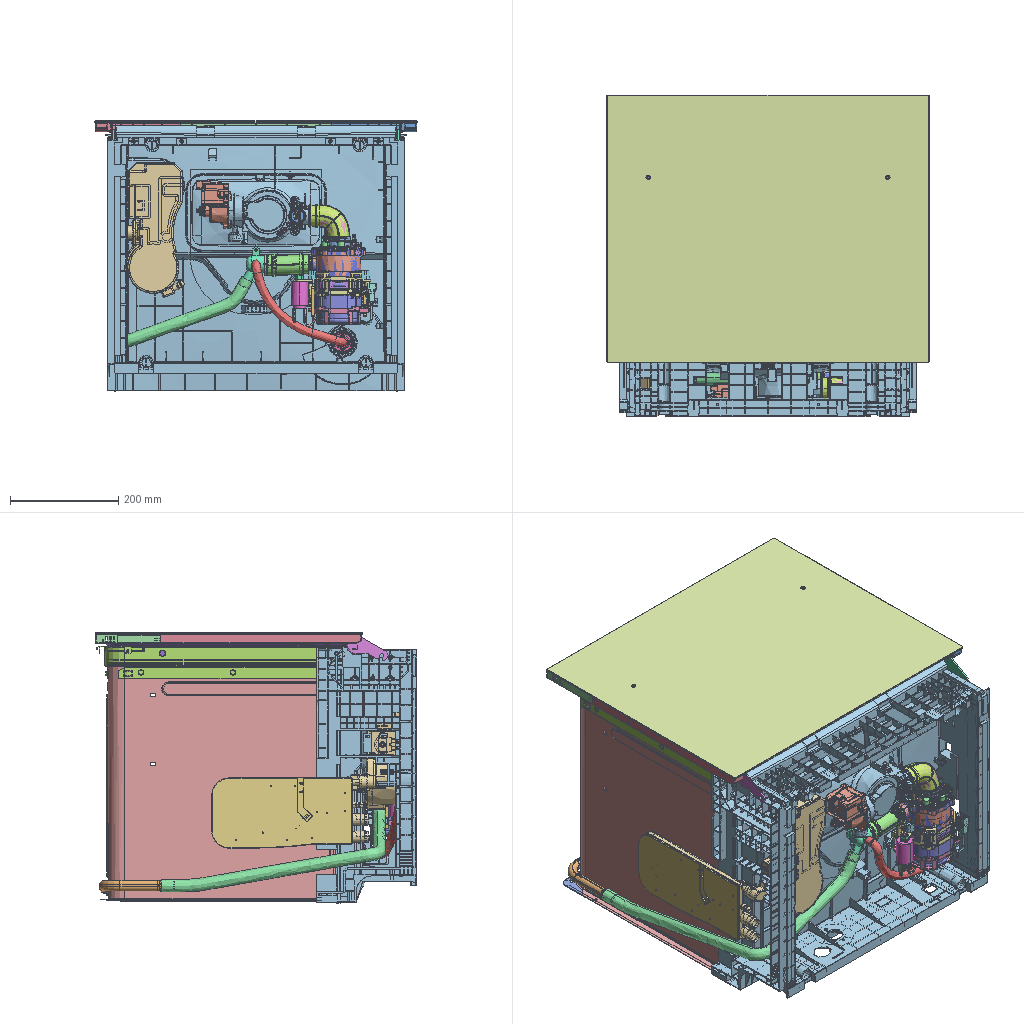Assembly | STEP file | 191 different items | 356 placed | box 596 x 594 x 500 mm
Parts list (item | name | quantity | parent item | size | volume):
1 | - | x1 | - | 3.8 x 3 x 1.2 mm | 13.052 mm3
2 | 12M0-U000-0002_A2512WRO-4P_1 | x1 | - | 12.48 x 9.8 x 8.57 mm | 221.308 mm3
3 | 12_12-3_5 | x1 | in BENGKEZUJIAN_ASM_29_ASM_1_ASM_1_ASM | 51.9 x 85 x 119.75 mm | 69599 mm3
4 | 19-HG_7_1 | x1 | in AC0410-190121_ASM_8_ASM_1_ASM | 112.641 x 83.966 x 33.2 mm | 28942 mm3
5 | 1903-QG_1 | x1 | in AC190301_ASM_2_ASM | 140.055 x 83.966 x 33 mm | 30398 mm3
6 | 8_20_3_1_1_14 | x1 | in BENGKEZUJIAN_ASM_29_ASM_1_ASM_1_ASM | 50.6 x 85 x 119.75 mm | 65552 mm3
7 | BENG1118_AF0_35_2_1_1 | x1 | in AC0410_ASM_9_ASM_6_ASM_3_ASM_1_ASM | 81.69 x 126.25 x 55 mm | 61777 mm3
8 | CHIWA_5_1_2_1_1 | x6 | in ZHUANZIZHUJIAN_ASM_9_1_ASM_1_AS_ASM | 18 x 11.5 x 2.4 mm | 490.68 mm3
9 | CIHUAN_7_1 | x1 | - | 34.75 x 20 x 34.75 mm | 14830 mm3
10 | DINGZITIEXING_8_1 | x1 | in ZHONGZHUANG_ASM_92_ASM_1_ASM | 73 x 15 x 73 mm | 38126 mm3
11 | DIZUO-XIN | x1 | in W721-DIZUO_ASM | - | 2428763 mm3
12 | DW-T1-02-0032_2_1_1 | x1 | in DW-T1-02-A004_ASM_1_ASM_2_ASM_1_ASM | 56 x 5.906 x 56 mm | 3121 mm3
13 | DW-T1-02-0033_2_6_1 | x1 | in DW-T1-02-A004_ASM_1_ASM_2_ASM_1_ASM | 56 x 19.052 x 56 mm | 7855 mm3
14 | DXDZ_1_1_1_1 | x1 | in AC0410_ASM_9_ASM_6_ASM_3_ASM_1_ASM | 8 x 16.965 x 7.531 mm | 100.473 mm3
15 | DZ250_3_1_1_1 | x2 | in AC0410_ASM_9_ASM_6_ASM_3_ASM_1_ASM | 8 x 13.602 x 13.602 mm | 104.298 mm3
16 | DZH_7_1 | x1 | - | 18.5 x 23 x 16 mm | 1219 mm3
17 | FANGHUALUOMAO_3_1 | x4 | in JIAREPANZUJIAN_ASM_76_ASM_2_ASM | 8 x 3.5 x 8 mm | 99.012 mm3
18 | GUANLU-XIAOPENBI | x1 | in 00-ZXW721_ASM_ASM | 176 x 160.5 x 71.93 mm | 30798 mm3
19 | HOUGAI_15_4 | x1 | in ZHONGZHUANG_ASM_92_ASM_1_ASM | 115 x 30 x 75 mm | 16947 mm3
20 | JAIREIPAN_146_1_1 | x1 | in JAIREIPAN_146_ASM_1_ASM | 99.5 x 85 x 6.5 mm | 5367 mm3
21 | JAIREIPAN_146_2_1 | x1 | in JAIREIPAN_146_ASM_1_ASM | 4.269 x 5.62 x 10.8 mm | 52.218 mm3
22 | JAIREIPAN_146_3_1 | x1 | in JAIREIPAN_146_ASM_1_ASM | 2.708 x 6.239 x 10.8 mm | 52.218 mm3
23 | JD20180502_ASM_1_ASM_2_1_1 | x1 | in DJ1118_ASM_5_ASM_4_ASM_7_ASM_1_ASM | - | -
24 | JD_1_1_1_1 | x2 | in DJ1118_ASM_5_ASM_4_ASM_7_ASM_1_ASM | 56 x 40 x 6 mm | 7974 mm3
25 | JIAREIGUAN_56_1 | x1 | in JIAREPANZUJIAN_ASM_76_ASM_2_ASM | 65 x 41.193 x 66.044 mm | 10951 mm3
26 | JIAREQI_2_1_1_1 | x1 | in AC0410_ASM_9_ASM_6_ASM_3_ASM_1_ASM | 62.5 x 63.088 x 35 mm | 12336 mm3
27 | LIANJIEQI1_17_1 | x1 | in ZHONGZHUANG_ASM_92_ASM_1_ASM | 19.4 x 30.7 x 11 mm | 1115 mm3
28 | LIANJIEQI2_14_1 | x1 | in ZHONGZHUANG_ASM_92_ASM_1_ASM | 20 x 23.5 x 10.5 mm | 729.279 mm3
29 | LUODING_1_1 | x6 | in JIAREPANZUJIAN_ASM_76_ASM_2_ASM | 6.44 x 6.44 x 10.399 mm | 92.165 mm3
30 | LUODING_1_1_1_1 | x4 | in DJ1118_ASM_5_ASM_4_ASM_7_ASM_1_ASM | - | -
31 | LUODING_5_1 | x3 | in ZHONGZHUANG_ASM_92_ASM_1_ASM | 5 x 14 x 5 mm | 98.522 mm3
32 | MIFENGQUAN1 | x1 | in 00-ZXW721_ASM_ASM | 19 x 19 x 3 mm | 355.306 mm3
33 | MIFENGQUAN2 | x1 | in 00-ZXW721_ASM_ASM | 28.5 x 28.5 x 2.6 mm | 525.838 mm3
34 | MIFENGQUAN_14_1_1_1 | x1 | in BENGKEZUJIAN_ASM_29_ASM_1_ASM_1_ASM | 81.15 x 81.15 x 2.65 mm | 1360 mm3
35 | MSBR-1 | x1 | in SHANGGEJIABAIFANG_ASM_ASM | 12.49 x 29.5 x 29.5 mm | 3348 mm3
36 | MSBR-10 | x1 | in SHANGGEJIABAIFANG_ASM_ASM | 12.49 x 29.5 x 29.5 mm | 3348 mm3
37 | MSBR-10_1_1_1_1 | x1 | in DJ1118_ASM_5_ASM_4_ASM_7_ASM_1_ASM | 7.904 x 7.691 x 3.2 mm | 92.564 mm3
38 | MSBR-11 | x1 | in SHANGGEJIABAIFANG_ASM_ASM | 26 x 13.7 x 15.65 mm | 1729 mm3
39 | MSBR-11_1_1_1_1 | x1 | in DJ1118_ASM_5_ASM_4_ASM_7_ASM_1_ASM | 7.691 x 7.904 x 3.2 mm | 92.564 mm3
40 | MSBR-12 | x1 | in SHANGGEJIABAIFANG_ASM_ASM | 12.744 x 31.5 x 31.5 mm | 3459 mm3
41 | MSBR-12_1_1_1_1 | x1 | in DJ1118_ASM_5_ASM_4_ASM_7_ASM_1_ASM | 7.904 x 7.691 x 3.2 mm | 92.564 mm3
42 | MSBR-13 | x1 | in SHANGGEJIABAIFANG_ASM_ASM | - | -
43 | MSBR-13_1_1_1_1 | x1 | in DJ1118_ASM_5_ASM_4_ASM_7_ASM_1_ASM | - | -
44 | MSBR-14 | x1 | in SHANGGEJIABAIFANG_ASM_ASM | 26 x 13.7 x 15.65 mm | 1729 mm3
45 | MSBR-14_1_1_1_1 | x1 | in DJ1118_ASM_5_ASM_4_ASM_7_ASM_1_ASM | 8.97 x 17.939 x 7.73 mm | 103.786 mm3
46 | MSBR-15 | x1 | in SHANGGEJIABAIFANG_ASM_ASM | 12.744 x 31.5 x 31.5 mm | 3459 mm3
47 | MSBR-15XIAO_2_1_1_1 | x8 | in AC0410_ASM_9_ASM_6_ASM_3_ASM_1_ASM | 6.44 x 6.44 x 10.399 mm | 92.165 mm3
48 | MSBR-15_1_1_1_1 | x1 | in DJ1118_ASM_5_ASM_4_ASM_7_ASM_1_ASM | 9.2 x 9.2 x 14.856 mm | 268.703 mm3
49 | MSBR-16 | x1 | in SHANGGEJIABAIFANG_ASM_ASM | - | -
50 | MSBR-16_1_5_4_1_1 | x1 | in MSBR-16_1_5_4_ASM_1_ASM | 34.276 x 35.044 x 77.065 mm | 5583 mm3
51 | MSBR-16_1_5_4_2_1 | x1 | in MSBR-16_1_5_4_ASM_1_ASM | 17.856 x 20.083 x 11.306 mm | 186.454 mm3
52 | MSBR-17 | x1 | in SHANGGEJIABAIFANG_ASM_ASM | 26 x 13.7 x 15.65 mm | 1729 mm3
53 | MSBR-17_1_1_1_1 | x1 | in DJ1118_ASM_5_ASM_4_ASM_7_ASM_1_ASM | 31 x 31 x 74.5 mm | 34990 mm3
54 | MSBR-18 | x1 | in SHANGGEJIABAIFANG_ASM_ASM | 12.744 x 31.5 x 31.5 mm | 3459 mm3
55 | MSBR-18_1_1_1_1 | x1 | in DJ1118_ASM_5_ASM_4_ASM_7_ASM_1_ASM | 21 x 21 x 0.5 mm | 84.823 mm3
56 | MSBR-19 | x1 | in SHANGGEJIABAIFANG_ASM_ASM | - | -
57 | MSBR-19_1_1_1_1 | x1 | in DJ1118_ASM_5_ASM_4_ASM_7_ASM_1_ASM | 21 x 21 x 0.5 mm | 84.823 mm3
58 | MSBR-1_7_1_1_1 | x1 | in DJ1118_ASM_5_ASM_4_ASM_7_ASM_1_ASM | - | -
59 | MSBR-2 | x1 | in SHANGGEJIABAIFANG_ASM_ASM | 26 x 13.7 x 15.65 mm | 1729 mm3
60 | MSBR-20 | x1 | in SHANGGEJIABAIFANG_ASM_ASM | 26 x 13.7 x 15.65 mm | 1729 mm3
61 | MSBR-20_1_1_1_1 | x1 | in DJ1118_ASM_5_ASM_4_ASM_7_ASM_1_ASM | 11.954 x 14 x 1 mm | 73.77 mm3
62 | MSBR-21 | x1 | in SHANGGEJIABAIFANG_ASM_ASM | 12.744 x 31.5 x 31.5 mm | 3459 mm3
63 | MSBR-21_1_1_1_1 | x1 | in DJ1118_ASM_5_ASM_4_ASM_7_ASM_1_ASM | 11.954 x 14 x 1 mm | 73.77 mm3
64 | MSBR-22 | x1 | in SHANGGEJIABAIFANG_ASM_ASM | - | -
65 | MSBR-22_1_1_1_1 | x1 | in DJ1118_ASM_5_ASM_4_ASM_7_ASM_1_ASM | 21.008 x 21.003 x 1.852 mm | 55.351 mm3
66 | MSBR-23 | x1 | in SHANGGEJIABAIFANG_ASM_ASM | 26 x 13.7 x 15.65 mm | 1729 mm3
67 | MSBR-23_1_1_1_1 | x1 | in DJ1118_ASM_5_ASM_4_ASM_7_ASM_1_ASM | 21.008 x 21.003 x 1.851 mm | 55.347 mm3
68 | MSBR-24 | x1 | in SHANGGEJIABAIFANG_ASM_ASM | 12.744 x 31.5 x 31.5 mm | 3459 mm3
69 | MSBR-25 | x1 | in SHANGGEJIABAIFANG_ASM_ASM | 43 x 43.4 x 205.2 mm | 28155 mm3
70 | MSBR-26 | x1 | in SHANGGEJIABAIFANG_ASM_ASM | 31 x 7.4 x 31 mm | 1482 mm3
71 | MSBR-27 | x1 | in SHANGGEJIABAIFANG_ASM_ASM | 31 x 1.2 x 31 mm | 268.606 mm3
72 | MSBR-28 | x1 | in SHANGGEJIABAIFANG_ASM_ASM | 415.551 x 17.694 x 58 mm | 32768 mm3
73 | MSBR-29 | x1 | in SHANGGEJIABAIFANG_ASM_ASM | 415.551 x 11.251 x 58 mm | 35121 mm3
74 | MSBR-2_1_1_1_1 | x1 | in DJ1118_ASM_5_ASM_4_ASM_7_ASM_1_ASM | 45.4 x 45.4 x 51 mm | 45376 mm3
75 | MSBR-3 | x1 | in SHANGGEJIABAIFANG_ASM_ASM | 12.744 x 31.5 x 31.5 mm | 3459 mm3
76 | MSBR-30 | x1 | in SHANGGEJIABAIFANG_ASM_ASM | - | -
77 | MSBR-31 | x1 | in SHANGGEJIABAIFANG_ASM_ASM | 55.5 x 13.7 x 53.411 mm | 7229 mm3
78 | MSBR-32 | x1 | in SHANGGEJIABAIFANG_ASM_ASM | 44 x 1 x 44 mm | 612.611 mm3
79 | MSBR-3_1_1_1_1 | x1 | in DJ1118_ASM_5_ASM_4_ASM_7_ASM_1_ASM | 22 x 22 x 7 mm | 2236 mm3
80 | MSBR-4 | x1 | in SHANGGEJIABAIFANG_ASM_ASM | 12.49 x 29.5 x 29.5 mm | 3348 mm3
81 | MSBR-4_1_1_1_1 | x1 | in DJ1118_ASM_5_ASM_4_ASM_7_ASM_1_ASM | 22 x 22 x 7 mm | 2236 mm3
82 | MSBR-5 | x1 | in SHANGGEJIABAIFANG_ASM_ASM | 26 x 13.7 x 15.65 mm | 1729 mm3
83 | MSBR-5_1_1_1_1 | x1 | in DJ1118_ASM_5_ASM_4_ASM_7_ASM_1_ASM | 84.5 x 84.5 x 74 mm | 208424 mm3
84 | MSBR-6 | x1 | in SHANGGEJIABAIFANG_ASM_ASM | 12.744 x 31.5 x 31.5 mm | 3459 mm3
85 | MSBR-6_1_1_1_1 | x1 | in DJ1118_ASM_5_ASM_4_ASM_7_ASM_1_ASM | 6.81 x 29.042 x 21.733 mm | 286.346 mm3
86 | MSBR-7 | x1 | in SHANGGEJIABAIFANG_ASM_ASM | 12.49 x 29.5 x 29.5 mm | 3348 mm3
87 | MSBR-8 | x1 | in SHANGGEJIABAIFANG_ASM_ASM | 26 x 13.7 x 15.65 mm | 1729 mm3
88 | MSBR-8_1_1_1_1 | x1 | in DJ1118_ASM_5_ASM_4_ASM_7_ASM_1_ASM | 13 x 14.856 x 6.8 mm | 647.005 mm3
89 | MSBR-9 | x1 | in SHANGGEJIABAIFANG_ASM_ASM | 12.744 x 31.5 x 31.5 mm | 3459 mm3
90 | MSBR-9_1_1_1_1 | x1 | in DJ1118_ASM_5_ASM_4_ASM_7_ASM_1_ASM | 7.691 x 7.904 x 3.2 mm | 92.564 mm3
91 | NCP18XH103F03RB_1 | x1 | - | 1.956 x 0.33 x 0.86 mm | 0.4616 mm3
92 | PINGBITAO_35_15 | x1 | in ZHUANZIZUJIAN_ASM_29_ASM_2_ASM | 114.5 x 53.2 x 85 mm | 39805 mm3
93 | PRT0001_20_1_1_1 | x1 | in YLZC_ASM_8_ASM_1_ASM_1_ASM_1_ASM | 56 x 56 x 20.61 mm | 7408 mm3
94 | PRT0008_6_1_2_3_2_1_1 | x2 | in SHIMOZHOUCHENZUJIAN_ASM_3_1_2_3_ASM | 7.5 x 10 x 10 mm | 432.724 mm3
95 | SHANGAI_7_1 | x1 | in ZHUANZIZUJIAN_ASM_29_ASM_2_ASM | 8.5 x 63.5 x 63.5 mm | 5943 mm3
96 | SHANGHUTAO_14_1 | x1 | in ZHONGZHUANG_ASM_92_ASM_1_ASM | 68 x 13.2 x 70 mm | 4829 mm3
97 | SHIMOZHOUCHENGWAITAO_6_1_2_3_2_ | x2 | in SHIMOZHOUCHENZUJIAN_ASM_3_1_2_3_ASM | 7 x 12 x 12 mm | 297.806 mm3
98 | TBS-1D91-0002_A0_O-RING_1 | x1 | in WENZHUOCHUANGANQI_ASM_ASM | 28.75 x 3.5 x 28.75 mm | 763.198 mm3
99 | - | x1 | - | 23 x 24.2 x 1.6 mm | 514.519 mm3
100 | TBS1006T_P9_W_1 | x1 | in WENZHUOCHUANGANQI_ASM_ASM | 46 x 30.115 x 12.1 mm | 2240 mm3
101 | TBS1007_P12_U_1 | x1 | in WENZHUOCHUANGANQI_ASM_ASM | 39.913 x 26.4 x 39.913 mm | 4035 mm3
102 | WENKONG1_2_1_1_1 | x2 | in AC0410_ASM_9_ASM_6_ASM_3_ASM_1_ASM | 16 x 15 x 22 mm | 1789 mm3
103 | WENKONG2_1_1_1_1 | x2 | in AC0410_ASM_9_ASM_6_ASM_3_ASM_1_ASM | 32 x 16 x 0.5 mm | 101.047 mm3
104 | WENKONGQI_16_1 | x2 | in WENKONGZHUJIAN_ASM_16_ASM_1_ASM | 17.2 x 19.8 x 15.8 mm | 2165 mm3
105 | WENKONGZHIJIA_3_1 | x2 | in WENKONGZHUJIAN_ASM_16_ASM_1_ASM | 17.7 x 3.2 x 33 mm | 72.757 mm3
106 | XIAHUTAO_29_1 | x1 | in ZHONGZHUANG_ASM_92_ASM_1_ASM | 68 x 23.3 x 70 mm | 5989 mm3
107 | XINAQUAN11_1_10_1 | x9 | in XINAQUAN11_1_ASM_1_ASM | 20.47 x 0.5 x 10.48 mm | 11.282 mm3
108 | XINAQUAN11_1_11_1 | x9 | in XINAQUAN11_1_ASM_1_ASM | 20.47 x 0.5 x 10.48 mm | 11.282 mm3
109 | XINAQUAN11_1_12_1 | x9 | in XINAQUAN11_1_ASM_1_ASM | 20.47 x 0.5 x 10.48 mm | 11.282 mm3
110 | XINAQUAN11_1_13_1 | x9 | in XINAQUAN11_1_ASM_1_ASM | 20.47 x 0.5 x 10.48 mm | 11.282 mm3
111 | XINAQUAN11_1_1_1 | x9 | in XINAQUAN11_1_ASM_1_ASM | 20.47 x 0.5 x 10.48 mm | 11.282 mm3
112 | XINAQUAN11_1_2_1 | x9 | in XINAQUAN11_1_ASM_1_ASM | 20.47 x 0.5 x 10.48 mm | 11.282 mm3
113 | XINAQUAN11_1_3_1 | x9 | in XINAQUAN11_1_ASM_1_ASM | 20.47 x 0.5 x 10.48 mm | 11.282 mm3
114 | XINAQUAN11_1_4_1 | x9 | in XINAQUAN11_1_ASM_1_ASM | 20.47 x 0.5 x 10.48 mm | 11.282 mm3
115 | XINAQUAN11_1_5_1 | x9 | in XINAQUAN11_1_ASM_1_ASM | 20.47 x 0.5 x 10.48 mm | 11.282 mm3
116 | XINAQUAN11_1_6_1 | x9 | in XINAQUAN11_1_ASM_1_ASM | 20.47 x 0.5 x 10.48 mm | 11.282 mm3
117 | XINAQUAN11_1_7_1 | x9 | in XINAQUAN11_1_ASM_1_ASM | 20.47 x 0.5 x 10.48 mm | 11.282 mm3
118 | XINAQUAN11_1_8_1 | x9 | in XINAQUAN11_1_ASM_1_ASM | 20.47 x 0.5 x 10.48 mm | 11.282 mm3
119 | XINAQUAN11_1_9_1 | x9 | in XINAQUAN11_1_ASM_1_ASM | 20.47 x 0.5 x 10.48 mm | 11.282 mm3
120 | YELUNDUTOU_8_1 | x1 | in YELUNZUJIAN_ASM_5_ASM_1_ASM | 12 x 20.5 x 12 mm | 1376 mm3
121 | YINGXIAN2_15_1 | x1 | in JIAREPANZUJIAN_ASM_76_ASM_2_ASM | 59.863 x 2 x 37.179 mm | 274.797 mm3
122 | YINGXIAN4_4_1 | x1 | in JIAREPANZUJIAN_ASM_76_ASM_2_ASM | 33.17 x 2 x 13.408 mm | 118.062 mm3
123 | YLG_9_1_1_1 | x1 | in YLZC_ASM_8_ASM_1_ASM_1_ASM_1_ASM | 56 x 56 x 9 mm | 3369 mm3
124 | ZHICHA_1_1_1 | x2 | in AC0410_ASM_9_ASM_6_ASM_3_ASM_1_ASM | 9.6 x 25.5 x 5.8 mm | 487.442 mm3
125 | ZHITUIZHOUCHEN_4_1_2_1_1 | x1 | in TUILIZHOUCHENGZUJIAN_ASM_2_1_AS_ASM | 3.7 x 17 x 17 mm | 365.454 mm3
126 | ZHOUTAO_18_1 | x1 | - | 28 x 24 x 28 mm | 4512 mm3
127 | ZHUANZHOU1_2_1_2_1_1 | x2 | in ZHUANZIZHUJIAN_ASM_9_1_ASM_1_AS_ASM | 62 x 5 x 5 mm | 1209 mm3
128 | ZHUANZITIEX_6_1_2_1_1 | x1 | in ZHUANZIZHUJIAN_ASM_9_1_ASM_1_AS_ASM | 15 x 25.116 x 27.5 mm | 6869 mm3
129 | ZHULVGAI_18_1_1_1 | x1 | in AC0410_ASM_9_ASM_6_ASM_3_ASM_1_ASM | 81.19 x 81 x 36 mm | 66134 mm3
130 | ZITUIZHOUCHEN2_3_1_2_1_1 | x1 | in TUILIZHOUCHENGZUJIAN_ASM_2_1_AS_ASM | 14.5 x 3.5 x 14.5 mm | 481.95 mm3
131 | ZUANZIWAITAO_4_1_2_1_1 | x1 | in ZHUANZIZHUJIAN_ASM_9_1_ASM_1_AS_ASM | 24.5 x 33 x 33 mm | 18261 mm3
132 | ZXCOMPANY_A722-L-147 | x1 | in ZXCOMPANY_A722-B-21_ASM | 117.864 x 121.275 x 6.608 mm | 9843 mm3
133 | ZXCOMPANY_A722-L-148 | x1 | in ZXCOMPANY_A722-B-21_ASM | 117.864 x 121.275 x 21.8 mm | 9245 mm3
134 | ZXCOMPANY_A722-L-149 | x1 | in XIAOPENBI_KAKOU-KAIYUAN_ASM | 36.755 x 40 x 33 mm | 6342 mm3
135 | ZXCOMPANY_A722-L-150 | x1 | in XIAOPENBI_KAKOU-KAIYUAN_ASM | 36 x 36 x 19.3 mm | 4496 mm3
136 | ZXCOMPANY_A782D-L-09 | x1 | in XIAOPENBI_KAKOU-KAIYUAN_ASM | 31.8 x 31.8 x 3 mm | 639.55 mm3
137 | ZXW722-L-01 | x1 | in W721-NEIDAN_ASM | 540.8 x 435.4 x 439.6 mm | 249280 mm3
138 | ZXW722-L-02 | x1 | in W721-NEIDAN_ASM | 540.8 x 435.4 x 4.2 mm | 101202 mm3
139 | ZXW722-L-03 | x1 | in W721-NEIDAN_ASM | 558 x 455.25 x 60 mm | 116020 mm3
140 | ZXW722-L-04 | x1 | in W721-NEIDAN_ASM | 47 x 12 x 4.9 mm | 258.28 mm3
141 | ZXW722-L-05 | x1 | in W721-MENTI_ASM | 596 x 494 x 3 mm | 882649 mm3
142 | ZXW722-L-10 | x1 | in W721-DIZUO_ASM | 249.6 x 15.181 x 134.6 mm | 18087 mm3
143 | ZXW722-L-11 | x1 | in W721-DIZUO_ASM | 82.99 x 80.1 x 65 mm | 13672 mm3
144 | ZXW722-L-13 | x1 | in W721-DIZUO_ASM | 39.088 x 46.093 x 29.8 mm | 5108 mm3
145 | ZXW722-L-15 | x1 | in ZXW722-B-03_ASM | 443.493 x 58 x 9.556 mm | 31671 mm3
146 | ZXW722-L-16 | x1 | in ZXW722-B-03_ASM | 443.493 x 58 x 51.016 mm | 34498 mm3
147 | ZXW722-L-178-B_21_1_1 | x1 | in ZXW722-B-06_20191205_ASM_52_1_A_ASM | 240.95 x 83.325 x 6.4 mm | 6922 mm3
148 | ZXW722-L-178-C_14_1_1 | x1 | in ZXW722-B-06_20191205_ASM_52_1_A_ASM | 421.95 x 80.725 x 6.4 mm | 12477 mm3
149 | ZXW722-L-178-D_23_1_1 | x1 | in ZXW722-B-06_20191205_ASM_52_1_A_ASM | 421.95 x 80.725 x 6.4 mm | 12477 mm3
150 | ZXW722-L-178_XIAGEJIA_19_1_2_1_ | x1 | in ZXW722-L-178_XIAGEJIA_19_1_2_AS_ASM | 487 x 185.95 x 459 mm | 160339 mm3
151 | ZXW722-L-178_XIAGEJIA_19_1_2_2_ | x1 | in ZXW722-L-178_XIAGEJIA_19_1_2_AS_ASM | 477.6 x 93 x 6.2 mm | 11029 mm3
152 | ZXW722-L-178_XIAGEJIA_19_1_2_3_ | x1 | in ZXW722-L-178_XIAGEJIA_19_1_2_AS_ASM | 477.6 x 93 x 25.9 mm | 11494 mm3
153 | ZXW722-L-19 | x1 | in W721-NEIDAN_ASM | 27.987 x 140.008 x 285 mm | 43724 mm3
154 | ZXW722-L-20 | x1 | in W721-NEIDAN_ASM | 39 x 135.5 x 59.4 mm | 32413 mm3
155 | ZXW722-L-21 | x1 | in W721-NEIDAN_ASM | 9.594 x 22.342 x 22.342 mm | 1117 mm3
156 | ZXW722-L-22 | x1 | in W721-NEIDAN_ASM | 30 x 20 x 30 mm | 5724 mm3
157 | ZXW722-L-24 | x1 | in W721-DIZUO_ASM | 84.8 x 86.614 x 84.8 mm | 30515 mm3
158 | ZXW722-L-25 | x1 | in W721-MENTI_ASM | 157.5 x 387 x 45.5 mm | 196671 mm3
159 | ZXW722-L-26 | x1 | in W721-MENTI_ASM | 157.5 x 387 x 45.5 mm | 196607 mm3
160 | ZXW722-L-27 | x1 | in W721-MENTI_ASM | 595 x 131 x 28.9 mm | 264991 mm3
161 | ZXW722-L-30 | x1 | in W721-MENTI_ASM | 547 x 485.1 x 31.6 mm | 126508 mm3
162 | ZXW722-L-31 | x1 | in W721-MENTI_ASM | 25.95 x 175.067 x 46.477 mm | 15631 mm3
163 | ZXW722-L-32 | x1 | in W721-MENTI_ASM | 25.95 x 175.067 x 46.477 mm | 15626 mm3
164 | ZXW722-L-35 | x1 | in W721-NEIDAN_ASM | 512.387 x 470.393 x 16.268 mm | 64395 mm3
165 | ZXW722-L-39 | x1 | in W721-DIZUO_ASM | 65.761 x 78.712 x 55.422 mm | 21689 mm3
166 | ZXW722-L-40 | x1 | in W721-DIZUO_ASM | 26.66 x 26.66 x 2.8 mm | 461.558 mm3
167 | ZXW722-L-50 | x1 | in W721-DIZUO_ASM | 36.029 x 65 x 32.601 mm | 13339 mm3
168 | ZXW722-L-57 | x1 | in 00-ZXW721_ASM_ASM | 268.527 x 414.68 x 191.423 mm | 152673 mm3
169 | ZXW722-L-76_SP | x1 | in W721-DIZUO_ASM | - | 2020809 mm3
170 | ZXW722-L-79-1 | x1 | in ZXW722-L-79_ASM | 10 x 22 x 23 mm | 593.01 mm3
171 | ZXW722-L-79-3 | x1 | in ZXW722-L-79_ASM | 7.9 x 7.9 x 2 mm | 58.231 mm3
172 | ZXW722-L-91 | x1 | in W722-DIANJI_ASM | 78.028 x 80.92 x 49.347 mm | 37026 mm3
173 | ZXW722-L-91_1_3_1 | x1 | - | 76.908 x 59.738 x 48.561 mm | 28536 mm3
174 | ZXW722-L-92 | x1 | in W722-DIANJI_ASM | 85 x 40.159 x 40.76 mm | 27832 mm3
175 | ZXW735-L-141_2_1_1 | x8 | in ZXW735-B-18_1_ASM_2_1_ASM_1_ASM | 14 x 35 x 35 mm | 4381 mm3
176 | ZXW735-L-142_1_2_1_1 | x8 | in ZXW735-B-18_1_ASM_2_1_ASM_1_ASM | 24.25 x 21.5 x 15 mm | 1561 mm3
177 | ZXW735-L-175_2_1_1 | x8 | in ZXW722-B-06_20191205_ASM_52_1_A_ASM | 29 x 13.5 x 12.958 mm | 1025 mm3
178 | ZXW735-L-178-A_11_1_1 | x1 | in ZXW722-B-06_20191205_ASM_52_1_A_ASM | 240.95 x 83.325 x 6.203 mm | 6917 mm3
179 | ZXW735-L-228_2_1_1 | x4 | in ZXW722-B-06_20191205_ASM_52_1_A_ASM | 8 x 23 x 8 mm | 701.957 mm3
180 | ZXW735-L-231_2_1_1 | x2 | in ZXW722-B-06_20191205_ASM_52_1_A_ASM | 32.5 x 27 x 42.902 mm | 6707 mm3
181 | ZXW735-L-232_2_1_1 | x2 | in ZXW722-B-06_20191205_ASM_52_1_A_ASM | 32.5 x 27 x 42.902 mm | 6709 mm3
182 | ZXW735-L-25 | x1 | in W721-DIZUO_ASM | 65 x 82.55 x 88.85 mm | 144092 mm3
183 | ZXW735-L-95-01 | x1 | in ZXW735-L-95_ASM | 28.6 x 23 x 44.35 mm | 7211 mm3
184 | ZXW735-L-95-02 | x1 | in ZXW735-L-95_ASM | 126.104 x 54.391 x 105.677 mm | 392404 mm3
185 | ZXW735-L-95-03 | x1 | in ZXW735-L-95_ASM | 36.6 x 13.445 x 108.794 mm | 27625 mm3
186 | ZXW735-L-95-04 | x1 | in ZXW735-L-95_ASM | 67.9 x 11.941 x 62.751 mm | 25948 mm3
187 | ZXW735-L-95-05 | x1 | in ZXW735-L-95_ASM | 14 x 9 x 8.417 mm | 278.257 mm3
188 | ZXW735-L-95-06 | x1 | in ZXW735-L-95_ASM | 125.904 x 7.7 x 105.477 mm | 15099 mm3
189 | _SHANGGEJIABAIFANG_ASM | x1 | in SHANGGEJIABAIFANG_ASM_ASM | - | -
190 | - | x1 | in JIAREPANZUJIAN_ASM_76_ASM_2_ASM | 40 x 20.98 x 40 mm | 3947 mm3
191 | - | x1 | - | 43 x 30.7 x 43 mm | 14945 mm3